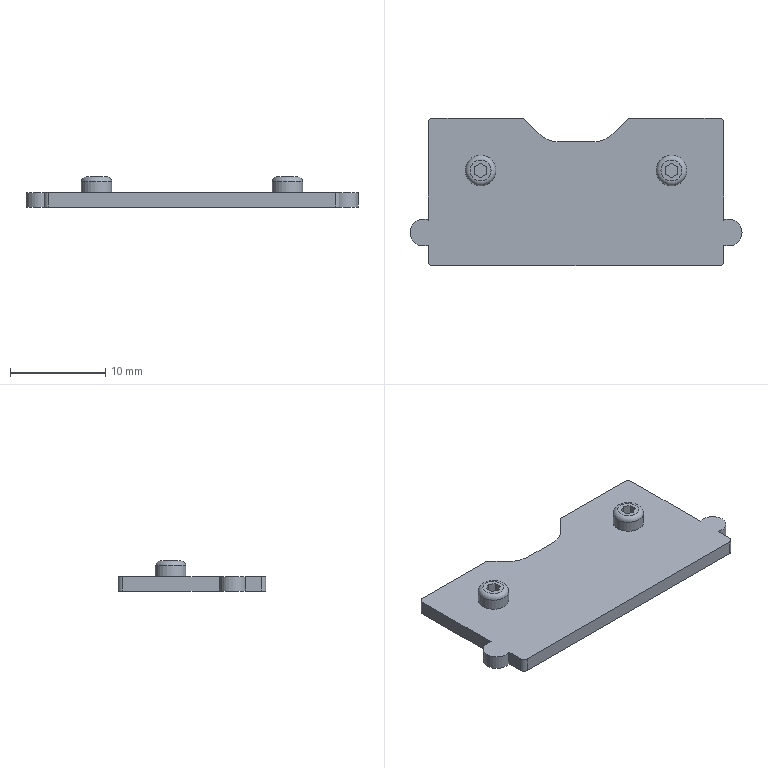Part | STEP file | BODY6_E-RAM6-S-640-ME30-C5 | 1 solid | 40 faces | box 34.8 x 15.5 x 3.15 mm | volume 724.972 mm3 | plane 28 | cylinder 10 | torus 2 | commonest cylinder face diameters 1 x4 2.8 x2 3.2 x2 6 x2
STEP:
#1=CARTESIAN_POINT('',(15.,5.5,1.5));
#2=VERTEX_POINT('',#1);
#3=CARTESIAN_POINT('',(5.5,5.5,1.5));
#4=VERTEX_POINT('',#3);
#5=CARTESIAN_POINT('',(-15.5,5.5,1.5));
#6=DIRECTION('',(-1.,0.,0.));
#7=VECTOR('',#6,1000.);
#8=LINE('',#5,#7);
#9=EDGE_CURVE('',#2,#4,#8,.T.);
#10=ORIENTED_EDGE('',*,*,#9,.F.);
#11=CARTESIAN_POINT('',(15.,5.5,0.));
#12=VERTEX_POINT('',#11);
#13=CARTESIAN_POINT('',(15.,5.5,1.5));
#14=DIRECTION('',(0.,0.,-1.));
#15=VECTOR('',#14,1000.);
#16=LINE('',#13,#15);
#17=EDGE_CURVE('',#2,#12,#16,.T.);
#18=ORIENTED_EDGE('',*,*,#17,.T.);
#19=CARTESIAN_POINT('',(5.5,5.5,0.));
#20=VERTEX_POINT('',#19);
#21=CARTESIAN_POINT('',(-15.5,5.5,0.));
#22=DIRECTION('',(-1.,0.,0.));
#23=VECTOR('',#22,1000.);
#24=LINE('',#21,#23);
#25=EDGE_CURVE('',#12,#20,#24,.T.);
#26=ORIENTED_EDGE('',*,*,#25,.T.);
#27=CARTESIAN_POINT('',(5.5,5.5,0.));
#28=DIRECTION('',(0.,0.,1.));
#29=VECTOR('',#28,1000.);
#30=LINE('',#27,#29);
#31=EDGE_CURVE('',#20,#4,#30,.T.);
#32=ORIENTED_EDGE('',*,*,#31,.T.);
#33=EDGE_LOOP('',(#10,#18,#26,#32));
#34=FACE_OUTER_BOUND('',#33,.T.);
#35=CARTESIAN_POINT('',(-15.5,5.5,1.5));
#36=DIRECTION('',(0.,-1.,0.));
#37=DIRECTION('',(0.,0.,-1.));
#38=AXIS2_PLACEMENT_3D('',#35,#36,#37);
#39=PLANE('',#38);
#40=ADVANCED_FACE('',(#34),#39,.F.);
#41=CARTESIAN_POINT('',(-15.5,-7.808,0.));
#42=VERTEX_POINT('',#41);
#43=CARTESIAN_POINT('',(-15.5,-9.5,0.));
#44=VERTEX_POINT('',#43);
#45=CARTESIAN_POINT('',(-15.5,-10.,0.));
#46=DIRECTION('',(0.,-1.,0.));
#47=VECTOR('',#46,1000.);
#48=LINE('',#45,#47);
#49=EDGE_CURVE('',#42,#44,#48,.T.);
#50=ORIENTED_EDGE('',*,*,#49,.T.);
#51=CARTESIAN_POINT('',(-15.5,-9.5,1.5));
#52=VERTEX_POINT('',#51);
#53=CARTESIAN_POINT('',(-15.5,-9.5,1.5));
#54=DIRECTION('',(0.,0.,1.));
#55=VECTOR('',#54,1000.);
#56=LINE('',#53,#55);
#57=EDGE_CURVE('',#44,#52,#56,.T.);
#58=ORIENTED_EDGE('',*,*,#57,.T.);
#59=CARTESIAN_POINT('',(-15.5,-7.808,1.5));
#60=VERTEX_POINT('',#59);
#61=CARTESIAN_POINT('',(-15.5,-10.,1.5));
#62=DIRECTION('',(0.,-1.,0.));
#63=VECTOR('',#62,1000.);
#64=LINE('',#61,#63);
#65=EDGE_CURVE('',#60,#52,#64,.T.);
#66=ORIENTED_EDGE('',*,*,#65,.F.);
#67=CARTESIAN_POINT('',(-15.5,-7.808,1.5));
#68=DIRECTION('',(0.,0.,-1.));
#69=VECTOR('',#68,1000.);
#70=LINE('',#67,#69);
#71=EDGE_CURVE('',#60,#42,#70,.T.);
#72=ORIENTED_EDGE('',*,*,#71,.T.);
#73=EDGE_LOOP('',(#50,#58,#66,#72));
#74=FACE_OUTER_BOUND('',#73,.T.);
#75=CARTESIAN_POINT('',(-15.5,-10.,1.5));
#76=DIRECTION('',(1.,0.,0.));
#77=DIRECTION('',(0.,0.,-1.));
#78=AXIS2_PLACEMENT_3D('',#75,#76,#77);
#79=PLANE('',#78);
#80=ADVANCED_FACE('',(#74),#79,.F.);
#81=CARTESIAN_POINT('',(-15.,-10.,0.));
#82=VERTEX_POINT('',#81);
#83=CARTESIAN_POINT('',(15.,-10.,0.));
#84=VERTEX_POINT('',#83);
#85=CARTESIAN_POINT('',(-15.5,-10.,0.));
#86=DIRECTION('',(1.,0.,0.));
#87=VECTOR('',#86,1000.);
#88=LINE('',#85,#87);
#89=EDGE_CURVE('',#82,#84,#88,.T.);
#90=ORIENTED_EDGE('',*,*,#89,.T.);
#91=CARTESIAN_POINT('',(15.,-10.,1.5));
#92=VERTEX_POINT('',#91);
#93=CARTESIAN_POINT('',(15.,-10.,1.5));
#94=DIRECTION('',(0.,0.,1.));
#95=VECTOR('',#94,1000.);
#96=LINE('',#93,#95);
#97=EDGE_CURVE('',#84,#92,#96,.T.);
#98=ORIENTED_EDGE('',*,*,#97,.T.);
#99=CARTESIAN_POINT('',(-15.,-10.,1.5));
#100=VERTEX_POINT('',#99);
#101=CARTESIAN_POINT('',(-15.5,-10.,1.5));
#102=DIRECTION('',(1.,0.,0.));
#103=VECTOR('',#102,1000.);
#104=LINE('',#101,#103);
#105=EDGE_CURVE('',#100,#92,#104,.T.);
#106=ORIENTED_EDGE('',*,*,#105,.F.);
#107=CARTESIAN_POINT('',(-15.,-10.,1.5));
#108=DIRECTION('',(0.,0.,-1.));
#109=VECTOR('',#108,1000.);
#110=LINE('',#107,#109);
#111=EDGE_CURVE('',#100,#82,#110,.T.);
#112=ORIENTED_EDGE('',*,*,#111,.T.);
#113=EDGE_LOOP('',(#90,#98,#106,#112));
#114=FACE_OUTER_BOUND('',#113,.T.);
#115=CARTESIAN_POINT('',(-15.5,-10.,1.5));
#116=DIRECTION('',(0.,1.,0.));
#117=DIRECTION('',(0.,0.,1.));
#118=AXIS2_PLACEMENT_3D('',#115,#116,#117);
#119=PLANE('',#118);
#120=ADVANCED_FACE('',(#114),#119,.F.);
#121=CARTESIAN_POINT('',(15.5,-9.5,1.5));
#122=VERTEX_POINT('',#121);
#123=CARTESIAN_POINT('',(15.5,-7.808,1.5));
#124=VERTEX_POINT('',#123);
#125=CARTESIAN_POINT('',(15.5,-10.,1.5));
#126=DIRECTION('',(0.,1.,0.));
#127=VECTOR('',#126,1000.);
#128=LINE('',#125,#127);
#129=EDGE_CURVE('',#122,#124,#128,.T.);
#130=ORIENTED_EDGE('',*,*,#129,.F.);
#131=CARTESIAN_POINT('',(15.5,-9.5,0.));
#132=VERTEX_POINT('',#131);
#133=CARTESIAN_POINT('',(15.5,-9.5,1.5));
#134=DIRECTION('',(0.,0.,-1.));
#135=VECTOR('',#134,1000.);
#136=LINE('',#133,#135);
#137=EDGE_CURVE('',#122,#132,#136,.T.);
#138=ORIENTED_EDGE('',*,*,#137,.T.);
#139=CARTESIAN_POINT('',(15.5,-7.808,0.));
#140=VERTEX_POINT('',#139);
#141=CARTESIAN_POINT('',(15.5,-10.,0.));
#142=DIRECTION('',(0.,1.,0.));
#143=VECTOR('',#142,1000.);
#144=LINE('',#141,#143);
#145=EDGE_CURVE('',#132,#140,#144,.T.);
#146=ORIENTED_EDGE('',*,*,#145,.T.);
#147=CARTESIAN_POINT('',(15.5,-7.808,1.5));
#148=DIRECTION('',(0.,0.,-1.));
#149=VECTOR('',#148,1000.);
#150=LINE('',#147,#149);
#151=EDGE_CURVE('',#124,#140,#150,.T.);
#152=ORIENTED_EDGE('',*,*,#151,.F.);
#153=EDGE_LOOP('',(#130,#138,#146,#152));
#154=FACE_OUTER_BOUND('',#153,.T.);
#155=CARTESIAN_POINT('',(15.5,-10.,1.5));
#156=DIRECTION('',(-1.,0.,0.));
#157=DIRECTION('',(0.,0.,1.));
#158=AXIS2_PLACEMENT_3D('',#155,#156,#157);
#159=PLANE('',#158);
#160=ADVANCED_FACE('',(#154),#159,.F.);
#161=CARTESIAN_POINT('',(15.5,-5.192,0.));
#162=VERTEX_POINT('',#161);
#163=CARTESIAN_POINT('',(16.,-6.5,0.));
#164=DIRECTION('',(0.,0.,1.));
#165=DIRECTION('',(1.,0.,0.));
#166=AXIS2_PLACEMENT_3D('',#163,#164,#165);
#167=CIRCLE('',#166,1.4);
#168=EDGE_CURVE('',#140,#162,#167,.T.);
#169=ORIENTED_EDGE('',*,*,#168,.T.);
#170=CARTESIAN_POINT('',(15.5,-5.192,1.5));
#171=VERTEX_POINT('',#170);
#172=CARTESIAN_POINT('',(15.5,-5.192,1.5));
#173=DIRECTION('',(0.,0.,-1.));
#174=VECTOR('',#173,1000.);
#175=LINE('',#172,#174);
#176=EDGE_CURVE('',#171,#162,#175,.T.);
#177=ORIENTED_EDGE('',*,*,#176,.F.);
#178=CARTESIAN_POINT('',(16.,-6.5,1.5));
#179=DIRECTION('',(0.,0.,1.));
#180=DIRECTION('',(1.,0.,0.));
#181=AXIS2_PLACEMENT_3D('',#178,#179,#180);
#182=CIRCLE('',#181,1.4);
#183=EDGE_CURVE('',#124,#171,#182,.T.);
#184=ORIENTED_EDGE('',*,*,#183,.F.);
#185=ORIENTED_EDGE('',*,*,#151,.T.);
#186=EDGE_LOOP('',(#169,#177,#184,#185));
#187=FACE_OUTER_BOUND('',#186,.T.);
#188=CARTESIAN_POINT('',(16.,-6.5,1.5));
#189=DIRECTION('',(0.,0.,-1.));
#190=DIRECTION('',(1.,0.,0.));
#191=AXIS2_PLACEMENT_3D('',#188,#189,#190);
#192=CYLINDRICAL_SURFACE('',#191,1.4);
#193=ADVANCED_FACE('',(#187),#192,.T.);
#194=CARTESIAN_POINT('',(15.5,5.,0.));
#195=VERTEX_POINT('',#194);
#196=CARTESIAN_POINT('',(15.5,-5.192,0.));
#197=DIRECTION('',(0.,1.,0.));
#198=VECTOR('',#197,1000.);
#199=LINE('',#196,#198);
#200=EDGE_CURVE('',#162,#195,#199,.T.);
#201=ORIENTED_EDGE('',*,*,#200,.T.);
#202=CARTESIAN_POINT('',(15.5,5.,1.5));
#203=VERTEX_POINT('',#202);
#204=CARTESIAN_POINT('',(15.5,5.,1.5));
#205=DIRECTION('',(0.,0.,1.));
#206=VECTOR('',#205,1000.);
#207=LINE('',#204,#206);
#208=EDGE_CURVE('',#195,#203,#207,.T.);
#209=ORIENTED_EDGE('',*,*,#208,.T.);
#210=CARTESIAN_POINT('',(15.5,-5.192,1.5));
#211=DIRECTION('',(0.,1.,0.));
#212=VECTOR('',#211,1000.);
#213=LINE('',#210,#212);
#214=EDGE_CURVE('',#171,#203,#213,.T.);
#215=ORIENTED_EDGE('',*,*,#214,.F.);
#216=ORIENTED_EDGE('',*,*,#176,.T.);
#217=EDGE_LOOP('',(#201,#209,#215,#216));
#218=FACE_OUTER_BOUND('',#217,.T.);
#219=CARTESIAN_POINT('',(15.5,-5.192,1.5));
#220=DIRECTION('',(-1.,0.,0.));
#221=DIRECTION('',(0.,0.,1.));
#222=AXIS2_PLACEMENT_3D('',#219,#220,#221);
#223=PLANE('',#222);
#224=ADVANCED_FACE('',(#218),#223,.F.);
#225=CARTESIAN_POINT('',(-5.5,5.5,0.));
#226=VERTEX_POINT('',#225);
#227=CARTESIAN_POINT('',(-15.,5.5,0.));
#228=VERTEX_POINT('',#227);
#229=CARTESIAN_POINT('',(-15.5,5.5,0.));
#230=DIRECTION('',(-1.,0.,0.));
#231=VECTOR('',#230,1000.);
#232=LINE('',#229,#231);
#233=EDGE_CURVE('',#226,#228,#232,.T.);
#234=ORIENTED_EDGE('',*,*,#233,.T.);
#235=CARTESIAN_POINT('',(-15.,5.5,1.5));
#236=VERTEX_POINT('',#235);
#237=CARTESIAN_POINT('',(-15.,5.5,1.5));
#238=DIRECTION('',(0.,0.,1.));
#239=VECTOR('',#238,1000.);
#240=LINE('',#237,#239);
#241=EDGE_CURVE('',#228,#236,#240,.T.);
#242=ORIENTED_EDGE('',*,*,#241,.T.);
#243=CARTESIAN_POINT('',(-5.5,5.5,1.5));
#244=VERTEX_POINT('',#243);
#245=CARTESIAN_POINT('',(-15.5,5.5,1.5));
#246=DIRECTION('',(-1.,0.,0.));
#247=VECTOR('',#246,1000.);
#248=LINE('',#245,#247);
#249=EDGE_CURVE('',#244,#236,#248,.T.);
#250=ORIENTED_EDGE('',*,*,#249,.F.);
#251=CARTESIAN_POINT('',(-5.5,5.5,0.));
#252=DIRECTION('',(0.,0.,1.));
#253=VECTOR('',#252,1000.);
#254=LINE('',#251,#253);
#255=EDGE_CURVE('',#226,#244,#254,.T.);
#256=ORIENTED_EDGE('',*,*,#255,.F.);
#257=EDGE_LOOP('',(#234,#242,#250,#256));
#258=FACE_OUTER_BOUND('',#257,.T.);
#259=CARTESIAN_POINT('',(-15.5,5.5,1.5));
#260=DIRECTION('',(0.,-1.,0.));
#261=DIRECTION('',(0.,0.,-1.));
#262=AXIS2_PLACEMENT_3D('',#259,#260,#261);
#263=PLANE('',#262);
#264=ADVANCED_FACE('',(#258),#263,.F.);
#265=CARTESIAN_POINT('',(-15.5,5.,1.5));
#266=VERTEX_POINT('',#265);
#267=CARTESIAN_POINT('',(-15.5,-5.192,1.5));
#268=VERTEX_POINT('',#267);
#269=CARTESIAN_POINT('',(-15.5,-5.192,1.5));
#270=DIRECTION('',(0.,-1.,0.));
#271=VECTOR('',#270,1000.);
#272=LINE('',#269,#271);
#273=EDGE_CURVE('',#266,#268,#272,.T.);
#274=ORIENTED_EDGE('',*,*,#273,.F.);
#275=CARTESIAN_POINT('',(-15.5,5.,0.));
#276=VERTEX_POINT('',#275);
#277=CARTESIAN_POINT('',(-15.5,5.,1.5));
#278=DIRECTION('',(0.,0.,-1.));
#279=VECTOR('',#278,1000.);
#280=LINE('',#277,#279);
#281=EDGE_CURVE('',#266,#276,#280,.T.);
#282=ORIENTED_EDGE('',*,*,#281,.T.);
#283=CARTESIAN_POINT('',(-15.5,-5.192,0.));
#284=VERTEX_POINT('',#283);
#285=CARTESIAN_POINT('',(-15.5,-5.192,0.));
#286=DIRECTION('',(0.,-1.,0.));
#287=VECTOR('',#286,1000.);
#288=LINE('',#285,#287);
#289=EDGE_CURVE('',#276,#284,#288,.T.);
#290=ORIENTED_EDGE('',*,*,#289,.T.);
#291=CARTESIAN_POINT('',(-15.5,-5.192,1.5));
#292=DIRECTION('',(0.,0.,-1.));
#293=VECTOR('',#292,1000.);
#294=LINE('',#291,#293);
#295=EDGE_CURVE('',#268,#284,#294,.T.);
#296=ORIENTED_EDGE('',*,*,#295,.F.);
#297=EDGE_LOOP('',(#274,#282,#290,#296));
#298=FACE_OUTER_BOUND('',#297,.T.);
#299=CARTESIAN_POINT('',(-15.5,-5.192,1.5));
#300=DIRECTION('',(1.,0.,0.));
#301=DIRECTION('',(0.,0.,-1.));
#302=AXIS2_PLACEMENT_3D('',#299,#300,#301);
#303=PLANE('',#302);
#304=ADVANCED_FACE('',(#298),#303,.F.);
#305=CARTESIAN_POINT('',(-16.,-6.5,0.));
#306=DIRECTION('',(0.,0.,1.));
#307=DIRECTION('',(1.,0.,0.));
#308=AXIS2_PLACEMENT_3D('',#305,#306,#307);
#309=CIRCLE('',#308,1.4);
#310=EDGE_CURVE('',#284,#42,#309,.T.);
#311=ORIENTED_EDGE('',*,*,#310,.T.);
#312=ORIENTED_EDGE('',*,*,#71,.F.);
#313=CARTESIAN_POINT('',(-16.,-6.5,1.5));
#314=DIRECTION('',(0.,0.,1.));
#315=DIRECTION('',(1.,0.,0.));
#316=AXIS2_PLACEMENT_3D('',#313,#314,#315);
#317=CIRCLE('',#316,1.4);
#318=EDGE_CURVE('',#268,#60,#317,.T.);
#319=ORIENTED_EDGE('',*,*,#318,.F.);
#320=ORIENTED_EDGE('',*,*,#295,.T.);
#321=EDGE_LOOP('',(#311,#312,#319,#320));
#322=FACE_OUTER_BOUND('',#321,.T.);
#323=CARTESIAN_POINT('',(-16.,-6.5,1.5));
#324=DIRECTION('',(0.,0.,-1.));
#325=DIRECTION('',(-1.,0.,0.));
#326=AXIS2_PLACEMENT_3D('',#323,#324,#325);
#327=CYLINDRICAL_SURFACE('',#326,1.4);
#328=ADVANCED_FACE('',(#322),#327,.T.);
#329=ORIENTED_EDGE('',*,*,#105,.T.);
#330=CARTESIAN_POINT('',(15.,-9.5,1.5));
#331=DIRECTION('',(0.,0.,1.));
#332=DIRECTION('',(1.,0.,0.));
#333=AXIS2_PLACEMENT_3D('',#330,#331,#332);
#334=CIRCLE('',#333,0.5);
#335=EDGE_CURVE('',#92,#122,#334,.T.);
#336=ORIENTED_EDGE('',*,*,#335,.T.);
#337=ORIENTED_EDGE('',*,*,#129,.T.);
#338=ORIENTED_EDGE('',*,*,#183,.T.);
#339=ORIENTED_EDGE('',*,*,#214,.T.);
#340=CARTESIAN_POINT('',(15.,5.,1.5));
#341=DIRECTION('',(0.,0.,1.));
#342=DIRECTION('',(1.,0.,0.));
#343=AXIS2_PLACEMENT_3D('',#340,#341,#342);
#344=CIRCLE('',#343,0.5);
#345=EDGE_CURVE('',#203,#2,#344,.T.);
#346=ORIENTED_EDGE('',*,*,#345,.T.);
#347=ORIENTED_EDGE('',*,*,#9,.T.);
#348=CARTESIAN_POINT('',(3.879,3.879,1.5));
#349=VERTEX_POINT('',#348);
#350=CARTESIAN_POINT('',(3.,3.,1.5));
#351=DIRECTION('',(0.7071,0.7071,0.));
#352=VECTOR('',#351,1000.);
#353=LINE('',#350,#352);
#354=EDGE_CURVE('',#349,#4,#353,.T.);
#355=ORIENTED_EDGE('',*,*,#354,.F.);
#356=CARTESIAN_POINT('',(1.757,3.,1.5));
#357=VERTEX_POINT('',#356);
#358=CARTESIAN_POINT('',(1.757,6.,1.5));
#359=DIRECTION('',(0.,0.,-1.));
#360=DIRECTION('',(1.,0.,0.));
#361=AXIS2_PLACEMENT_3D('',#358,#359,#360);
#362=CIRCLE('',#361,3.);
#363=EDGE_CURVE('',#349,#357,#362,.T.);
#364=ORIENTED_EDGE('',*,*,#363,.T.);
#365=CARTESIAN_POINT('',(-1.757,3.,1.5));
#366=VERTEX_POINT('',#365);
#367=CARTESIAN_POINT('',(-3.,3.,1.5));
#368=DIRECTION('',(1.,0.,0.));
#369=VECTOR('',#368,1000.);
#370=LINE('',#367,#369);
#371=EDGE_CURVE('',#366,#357,#370,.T.);
#372=ORIENTED_EDGE('',*,*,#371,.F.);
#373=CARTESIAN_POINT('',(-3.879,3.879,1.5));
#374=VERTEX_POINT('',#373);
#375=CARTESIAN_POINT('',(-1.757,6.,1.5));
#376=DIRECTION('',(0.,0.,-1.));
#377=DIRECTION('',(1.,0.,0.));
#378=AXIS2_PLACEMENT_3D('',#375,#376,#377);
#379=CIRCLE('',#378,3.);
#380=EDGE_CURVE('',#366,#374,#379,.T.);
#381=ORIENTED_EDGE('',*,*,#380,.T.);
#382=CARTESIAN_POINT('',(-5.5,5.5,1.5));
#383=DIRECTION('',(0.7071,-0.7071,0.));
#384=VECTOR('',#383,1000.);
#385=LINE('',#382,#384);
#386=EDGE_CURVE('',#244,#374,#385,.T.);
#387=ORIENTED_EDGE('',*,*,#386,.F.);
#388=ORIENTED_EDGE('',*,*,#249,.T.);
#389=CARTESIAN_POINT('',(-15.,5.,1.5));
#390=DIRECTION('',(0.,0.,1.));
#391=DIRECTION('',(1.,0.,0.));
#392=AXIS2_PLACEMENT_3D('',#389,#390,#391);
#393=CIRCLE('',#392,0.5);
#394=EDGE_CURVE('',#236,#266,#393,.T.);
#395=ORIENTED_EDGE('',*,*,#394,.T.);
#396=ORIENTED_EDGE('',*,*,#273,.T.);
#397=ORIENTED_EDGE('',*,*,#318,.T.);
#398=ORIENTED_EDGE('',*,*,#65,.T.);
#399=CARTESIAN_POINT('',(-15.,-9.5,1.5));
#400=DIRECTION('',(0.,0.,1.));
#401=DIRECTION('',(1.,0.,0.));
#402=AXIS2_PLACEMENT_3D('',#399,#400,#401);
#403=CIRCLE('',#402,0.5);
#404=EDGE_CURVE('',#52,#100,#403,.T.);
#405=ORIENTED_EDGE('',*,*,#404,.T.);
#406=EDGE_LOOP('',(#329,#336,#337,#338,#339,#346,#347,#355,#364,#372,#381,#387,#388,#395,#396,#397,#398,#405));
#407=FACE_OUTER_BOUND('',#406,.T.);
#408=CARTESIAN_POINT('',(11.6,0.,1.5));
#409=VERTEX_POINT('',#408);
#410=CARTESIAN_POINT('',(10.,0.,1.5));
#411=DIRECTION('',(0.,0.,1.));
#412=DIRECTION('',(1.,0.,0.));
#413=AXIS2_PLACEMENT_3D('',#410,#411,#412);
#414=CIRCLE('',#413,1.6);
#415=EDGE_CURVE('',#409,#409,#414,.T.);
#416=ORIENTED_EDGE('',*,*,#415,.F.);
#417=EDGE_LOOP('',(#416));
#418=FACE_BOUND('',#417,.T.);
#419=CARTESIAN_POINT('',(-8.4,0.,1.5));
#420=VERTEX_POINT('',#419);
#421=CARTESIAN_POINT('',(-10.,0.,1.5));
#422=DIRECTION('',(0.,0.,1.));
#423=DIRECTION('',(1.,0.,0.));
#424=AXIS2_PLACEMENT_3D('',#421,#422,#423);
#425=CIRCLE('',#424,1.6);
#426=EDGE_CURVE('',#420,#420,#425,.T.);
#427=ORIENTED_EDGE('',*,*,#426,.F.);
#428=EDGE_LOOP('',(#427));
#429=FACE_BOUND('',#428,.T.);
#430=CARTESIAN_POINT('',(-16.,-6.5,1.5));
#431=DIRECTION('',(0.,0.,1.));
#432=DIRECTION('',(1.,0.,0.));
#433=AXIS2_PLACEMENT_3D('',#430,#431,#432);
#434=PLANE('',#433);
#435=ADVANCED_FACE('',(#407,#418,#429),#434,.T.);
#436=ORIENTED_EDGE('',*,*,#145,.F.);
#437=CARTESIAN_POINT('',(15.,-9.5,0.));
#438=DIRECTION('',(0.,0.,-1.));
#439=DIRECTION('',(1.,0.,0.));
#440=AXIS2_PLACEMENT_3D('',#437,#438,#439);
#441=CIRCLE('',#440,0.5);
#442=EDGE_CURVE('',#132,#84,#441,.T.);
#443=ORIENTED_EDGE('',*,*,#442,.T.);
#444=ORIENTED_EDGE('',*,*,#89,.F.);
#445=CARTESIAN_POINT('',(-15.,-9.5,0.));
#446=DIRECTION('',(0.,0.,-1.));
#447=DIRECTION('',(1.,0.,0.));
#448=AXIS2_PLACEMENT_3D('',#445,#446,#447);
#449=CIRCLE('',#448,0.5);
#450=EDGE_CURVE('',#82,#44,#449,.T.);
#451=ORIENTED_EDGE('',*,*,#450,.T.);
#452=ORIENTED_EDGE('',*,*,#49,.F.);
#453=ORIENTED_EDGE('',*,*,#310,.F.);
#454=ORIENTED_EDGE('',*,*,#289,.F.);
#455=CARTESIAN_POINT('',(-15.,5.,0.));
#456=DIRECTION('',(0.,0.,-1.));
#457=DIRECTION('',(1.,0.,0.));
#458=AXIS2_PLACEMENT_3D('',#455,#456,#457);
#459=CIRCLE('',#458,0.5);
#460=EDGE_CURVE('',#276,#228,#459,.T.);
#461=ORIENTED_EDGE('',*,*,#460,.T.);
#462=ORIENTED_EDGE('',*,*,#233,.F.);
#463=CARTESIAN_POINT('',(-3.879,3.879,0.));
#464=VERTEX_POINT('',#463);
#465=CARTESIAN_POINT('',(-5.5,5.5,0.));
#466=DIRECTION('',(0.7071,-0.7071,0.));
#467=VECTOR('',#466,1000.);
#468=LINE('',#465,#467);
#469=EDGE_CURVE('',#226,#464,#468,.T.);
#470=ORIENTED_EDGE('',*,*,#469,.T.);
#471=CARTESIAN_POINT('',(-1.757,3.,0.));
#472=VERTEX_POINT('',#471);
#473=CARTESIAN_POINT('',(-1.757,6.,0.));
#474=DIRECTION('',(0.,0.,1.));
#475=DIRECTION('',(1.,0.,0.));
#476=AXIS2_PLACEMENT_3D('',#473,#474,#475);
#477=CIRCLE('',#476,3.);
#478=EDGE_CURVE('',#464,#472,#477,.T.);
#479=ORIENTED_EDGE('',*,*,#478,.T.);
#480=CARTESIAN_POINT('',(1.757,3.,0.));
#481=VERTEX_POINT('',#480);
#482=CARTESIAN_POINT('',(-3.,3.,0.));
#483=DIRECTION('',(1.,0.,0.));
#484=VECTOR('',#483,1000.);
#485=LINE('',#482,#484);
#486=EDGE_CURVE('',#472,#481,#485,.T.);
#487=ORIENTED_EDGE('',*,*,#486,.T.);
#488=CARTESIAN_POINT('',(3.879,3.879,0.));
#489=VERTEX_POINT('',#488);
#490=CARTESIAN_POINT('',(1.757,6.,0.));
#491=DIRECTION('',(0.,0.,1.));
#492=DIRECTION('',(1.,0.,0.));
#493=AXIS2_PLACEMENT_3D('',#490,#491,#492);
#494=CIRCLE('',#493,3.);
#495=EDGE_CURVE('',#481,#489,#494,.T.);
#496=ORIENTED_EDGE('',*,*,#495,.T.);
#497=CARTESIAN_POINT('',(3.,3.,0.));
#498=DIRECTION('',(0.7071,0.7071,0.));
#499=VECTOR('',#498,1000.);
#500=LINE('',#497,#499);
#501=EDGE_CURVE('',#489,#20,#500,.T.);
#502=ORIENTED_EDGE('',*,*,#501,.T.);
#503=ORIENTED_EDGE('',*,*,#25,.F.);
#504=CARTESIAN_POINT('',(15.,5.,0.));
#505=DIRECTION('',(0.,0.,-1.));
#506=DIRECTION('',(1.,0.,0.));
#507=AXIS2_PLACEMENT_3D('',#504,#505,#506);
#508=CIRCLE('',#507,0.5);
#509=EDGE_CURVE('',#12,#195,#508,.T.);
#510=ORIENTED_EDGE('',*,*,#509,.T.);
#511=ORIENTED_EDGE('',*,*,#200,.F.);
#512=ORIENTED_EDGE('',*,*,#168,.F.);
#513=EDGE_LOOP('',(#436,#443,#444,#451,#452,#453,#454,#461,#462,#470,#479,#487,#496,#502,#503,#510,#511,#512));
#514=FACE_OUTER_BOUND('',#513,.T.);
#515=CARTESIAN_POINT('',(-16.,-6.5,0.));
#516=DIRECTION('',(0.,0.,1.));
#517=DIRECTION('',(1.,0.,0.));
#518=AXIS2_PLACEMENT_3D('',#515,#516,#517);
#519=PLANE('',#518);
#520=ADVANCED_FACE('',(#514),#519,.F.);
#521=ORIENTED_EDGE('',*,*,#426,.T.);
#522=CARTESIAN_POINT('',(-8.4,0.,2.65));
#523=VERTEX_POINT('',#522);
#524=CARTESIAN_POINT('',(-8.4,0.,3.15));
#525=DIRECTION('',(0.,0.,1.));
#526=VECTOR('',#525,1.6);
#527=LINE('',#524,#526);
#528=EDGE_CURVE('',#420,#523,#527,.T.);
#529=ORIENTED_EDGE('',*,*,#528,.T.);
#530=CARTESIAN_POINT('',(-11.6,0.,2.65));
#531=VERTEX_POINT('',#530);
#532=CARTESIAN_POINT('',(-10.,0.,2.65));
#533=DIRECTION('',(0.,0.,-1.));
#534=DIRECTION('',(1.,0.,0.));
#535=AXIS2_PLACEMENT_3D('',#532,#533,#534);
#536=CIRCLE('',#535,1.6);
#537=EDGE_CURVE('',#523,#531,#536,.T.);
#538=ORIENTED_EDGE('',*,*,#537,.T.);
#539=CARTESIAN_POINT('',(-10.,0.,2.65));
#540=DIRECTION('',(0.,0.,-1.));
#541=DIRECTION('',(1.,0.,0.));
#542=AXIS2_PLACEMENT_3D('',#539,#540,#541);
#543=CIRCLE('',#542,1.6);
#544=EDGE_CURVE('',#531,#523,#543,.T.);
#545=ORIENTED_EDGE('',*,*,#544,.T.);
#546=ORIENTED_EDGE('',*,*,#528,.F.);
#547=EDGE_LOOP('',(#521,#529,#538,#545,#546));
#548=FACE_OUTER_BOUND('',#547,.T.);
#549=CARTESIAN_POINT('',(-10.,0.,3.15));
#550=DIRECTION('',(0.,0.,-1.));
#551=DIRECTION('',(-1.,0.,0.));
#552=AXIS2_PLACEMENT_3D('',#549,#550,#551);
#553=CYLINDRICAL_SURFACE('',#552,1.6);
#554=ADVANCED_FACE('',(#548),#553,.T.);
#555=CARTESIAN_POINT('',(-8.9,0.,3.15));
#556=VERTEX_POINT('',#555);
#557=CARTESIAN_POINT('',(-11.1,0.,3.15));
#558=VERTEX_POINT('',#557);
#559=CARTESIAN_POINT('',(-10.,0.,3.15));
#560=DIRECTION('',(0.,0.,1.));
#561=DIRECTION('',(1.,0.,0.));
#562=AXIS2_PLACEMENT_3D('',#559,#560,#561);
#563=CIRCLE('',#562,1.1);
#564=EDGE_CURVE('',#556,#558,#563,.T.);
#565=ORIENTED_EDGE('',*,*,#564,.T.);
#566=CARTESIAN_POINT('',(-10.,0.,3.15));
#567=DIRECTION('',(0.,0.,1.));
#568=DIRECTION('',(1.,0.,0.));
#569=AXIS2_PLACEMENT_3D('',#566,#567,#568);
#570=CIRCLE('',#569,1.1);
#571=EDGE_CURVE('',#558,#556,#570,.T.);
#572=ORIENTED_EDGE('',*,*,#571,.T.);
#573=EDGE_LOOP('',(#565,#572));
#574=FACE_OUTER_BOUND('',#573,.T.);
#575=CARTESIAN_POINT('',(-9.35,0.3753,3.15));
#576=VERTEX_POINT('',#575);
#577=CARTESIAN_POINT('',(-10.,0.7506,3.15));
#578=VERTEX_POINT('',#577);
#579=CARTESIAN_POINT('',(-9.35,0.3753,3.15));
#580=DIRECTION('',(-0.866,0.5,0.));
#581=VECTOR('',#580,1000.);
#582=LINE('',#579,#581);
#583=EDGE_CURVE('',#576,#578,#582,.T.);
#584=ORIENTED_EDGE('',*,*,#583,.F.);
#585=CARTESIAN_POINT('',(-9.35,-0.3753,3.15));
#586=VERTEX_POINT('',#585);
#587=CARTESIAN_POINT('',(-9.35,-0.3753,3.15));
#588=DIRECTION('',(0.,1.,0.));
#589=VECTOR('',#588,1000.);
#590=LINE('',#587,#589);
#591=EDGE_CURVE('',#586,#576,#590,.T.);
#592=ORIENTED_EDGE('',*,*,#591,.F.);
#593=CARTESIAN_POINT('',(-10.,-0.7506,3.15));
#594=VERTEX_POINT('',#593);
#595=CARTESIAN_POINT('',(-10.,-0.7506,3.15));
#596=DIRECTION('',(0.866,0.5,0.));
#597=VECTOR('',#596,1000.);
#598=LINE('',#595,#597);
#599=EDGE_CURVE('',#594,#586,#598,.T.);
#600=ORIENTED_EDGE('',*,*,#599,.F.);
#601=CARTESIAN_POINT('',(-10.65,-0.3753,3.15));
#602=VERTEX_POINT('',#601);
#603=CARTESIAN_POINT('',(-10.65,-0.3753,3.15));
#604=DIRECTION('',(0.866,-0.5,0.));
#605=VECTOR('',#604,1000.);
#606=LINE('',#603,#605);
#607=EDGE_CURVE('',#602,#594,#606,.T.);
#608=ORIENTED_EDGE('',*,*,#607,.F.);
#609=CARTESIAN_POINT('',(-10.65,0.3753,3.15));
#610=VERTEX_POINT('',#609);
#611=CARTESIAN_POINT('',(-10.65,0.3753,3.15));
#612=DIRECTION('',(0.,-1.,0.));
#613=VECTOR('',#612,1000.);
#614=LINE('',#611,#613);
#615=EDGE_CURVE('',#610,#602,#614,.T.);
#616=ORIENTED_EDGE('',*,*,#615,.F.);
#617=CARTESIAN_POINT('',(-10.,0.7506,3.15));
#618=DIRECTION('',(-0.866,-0.5,0.));
#619=VECTOR('',#618,1000.);
#620=LINE('',#617,#619);
#621=EDGE_CURVE('',#578,#610,#620,.T.);
#622=ORIENTED_EDGE('',*,*,#621,.F.);
#623=EDGE_LOOP('',(#584,#592,#600,#608,#616,#622));
#624=FACE_BOUND('',#623,.T.);
#625=CARTESIAN_POINT('',(-10.,0.,3.15));
#626=DIRECTION('',(0.,0.,1.));
#627=DIRECTION('',(1.,0.,0.));
#628=AXIS2_PLACEMENT_3D('',#625,#626,#627);
#629=PLANE('',#628);
#630=ADVANCED_FACE('',(#574,#624),#629,.T.);
#631=ORIENTED_EDGE('',*,*,#415,.T.);
#632=CARTESIAN_POINT('',(11.6,0.,2.65));
#633=VERTEX_POINT('',#632);
#634=CARTESIAN_POINT('',(11.6,0.,3.15));
#635=DIRECTION('',(0.,0.,1.));
#636=VECTOR('',#635,1.6);
#637=LINE('',#634,#636);
#638=EDGE_CURVE('',#409,#633,#637,.T.);
#639=ORIENTED_EDGE('',*,*,#638,.T.);
#640=CARTESIAN_POINT('',(8.4,0.,2.65));
#641=VERTEX_POINT('',#640);
#642=CARTESIAN_POINT('',(10.,0.,2.65));
#643=DIRECTION('',(0.,0.,-1.));
#644=DIRECTION('',(1.,0.,0.));
#645=AXIS2_PLACEMENT_3D('',#642,#643,#644);
#646=CIRCLE('',#645,1.6);
#647=EDGE_CURVE('',#633,#641,#646,.T.);
#648=ORIENTED_EDGE('',*,*,#647,.T.);
#649=CARTESIAN_POINT('',(10.,0.,2.65));
#650=DIRECTION('',(0.,0.,-1.));
#651=DIRECTION('',(1.,0.,0.));
#652=AXIS2_PLACEMENT_3D('',#649,#650,#651);
#653=CIRCLE('',#652,1.6);
#654=EDGE_CURVE('',#641,#633,#653,.T.);
#655=ORIENTED_EDGE('',*,*,#654,.T.);
#656=ORIENTED_EDGE('',*,*,#638,.F.);
#657=EDGE_LOOP('',(#631,#639,#648,#655,#656));
#658=FACE_OUTER_BOUND('',#657,.T.);
#659=CARTESIAN_POINT('',(10.,0.,3.15));
#660=DIRECTION('',(0.,0.,-1.));
#661=DIRECTION('',(-1.,0.,0.));
#662=AXIS2_PLACEMENT_3D('',#659,#660,#661);
#663=CYLINDRICAL_SURFACE('',#662,1.6);
#664=ADVANCED_FACE('',(#658),#663,.T.);
#665=CARTESIAN_POINT('',(11.1,0.,3.15));
#666=VERTEX_POINT('',#665);
#667=CARTESIAN_POINT('',(8.9,0.,3.15));
#668=VERTEX_POINT('',#667);
#669=CARTESIAN_POINT('',(10.,0.,3.15));
#670=DIRECTION('',(0.,0.,1.));
#671=DIRECTION('',(1.,0.,0.));
#672=AXIS2_PLACEMENT_3D('',#669,#670,#671);
#673=CIRCLE('',#672,1.1);
#674=EDGE_CURVE('',#666,#668,#673,.T.);
#675=ORIENTED_EDGE('',*,*,#674,.T.);
#676=CARTESIAN_POINT('',(10.,0.,3.15));
#677=DIRECTION('',(0.,0.,1.));
#678=DIRECTION('',(1.,0.,0.));
#679=AXIS2_PLACEMENT_3D('',#676,#677,#678);
#680=CIRCLE('',#679,1.1);
#681=EDGE_CURVE('',#668,#666,#680,.T.);
#682=ORIENTED_EDGE('',*,*,#681,.T.);
#683=EDGE_LOOP('',(#675,#682));
#684=FACE_OUTER_BOUND('',#683,.T.);
#685=CARTESIAN_POINT('',(10.65,0.3753,3.15));
#686=VERTEX_POINT('',#685);
#687=CARTESIAN_POINT('',(10.,0.7506,3.15));
#688=VERTEX_POINT('',#687);
#689=CARTESIAN_POINT('',(10.65,0.3753,3.15));
#690=DIRECTION('',(-0.866,0.5,0.));
#691=VECTOR('',#690,1000.);
#692=LINE('',#689,#691);
#693=EDGE_CURVE('',#686,#688,#692,.T.);
#694=ORIENTED_EDGE('',*,*,#693,.F.);
#695=CARTESIAN_POINT('',(10.65,-0.3753,3.15));
#696=VERTEX_POINT('',#695);
#697=CARTESIAN_POINT('',(10.65,-0.3753,3.15));
#698=DIRECTION('',(0.,1.,0.));
#699=VECTOR('',#698,1000.);
#700=LINE('',#697,#699);
#701=EDGE_CURVE('',#696,#686,#700,.T.);
#702=ORIENTED_EDGE('',*,*,#701,.F.);
#703=CARTESIAN_POINT('',(10.,-0.7506,3.15));
#704=VERTEX_POINT('',#703);
#705=CARTESIAN_POINT('',(10.,-0.7506,3.15));
#706=DIRECTION('',(0.866,0.5,0.));
#707=VECTOR('',#706,1000.);
#708=LINE('',#705,#707);
#709=EDGE_CURVE('',#704,#696,#708,.T.);
#710=ORIENTED_EDGE('',*,*,#709,.F.);
#711=CARTESIAN_POINT('',(9.35,-0.3753,3.15));
#712=VERTEX_POINT('',#711);
#713=CARTESIAN_POINT('',(9.35,-0.3753,3.15));
#714=DIRECTION('',(0.866,-0.5,0.));
#715=VECTOR('',#714,1000.);
#716=LINE('',#713,#715);
#717=EDGE_CURVE('',#712,#704,#716,.T.);
#718=ORIENTED_EDGE('',*,*,#717,.F.);
#719=CARTESIAN_POINT('',(9.35,0.3753,3.15));
#720=VERTEX_POINT('',#719);
#721=CARTESIAN_POINT('',(9.35,0.3753,3.15));
#722=DIRECTION('',(0.,-1.,0.));
#723=VECTOR('',#722,1000.);
#724=LINE('',#721,#723);
#725=EDGE_CURVE('',#720,#712,#724,.T.);
#726=ORIENTED_EDGE('',*,*,#725,.F.);
#727=CARTESIAN_POINT('',(10.,0.7506,3.15));
#728=DIRECTION('',(-0.866,-0.5,0.));
#729=VECTOR('',#728,1000.);
#730=LINE('',#727,#729);
#731=EDGE_CURVE('',#688,#720,#730,.T.);
#732=ORIENTED_EDGE('',*,*,#731,.F.);
#733=EDGE_LOOP('',(#694,#702,#710,#718,#726,#732));
#734=FACE_BOUND('',#733,.T.);
#735=CARTESIAN_POINT('',(10.,0.,3.15));
#736=DIRECTION('',(0.,0.,1.));
#737=DIRECTION('',(1.,0.,0.));
#738=AXIS2_PLACEMENT_3D('',#735,#736,#737);
#739=PLANE('',#738);
#740=ADVANCED_FACE('',(#684,#734),#739,.T.);
#741=ORIENTED_EDGE('',*,*,#583,.T.);
#742=CARTESIAN_POINT('',(-10.,0.7506,2.11));
#743=VERTEX_POINT('',#742);
#744=CARTESIAN_POINT('',(-10.,0.7506,2.11));
#745=DIRECTION('',(0.,0.,1.));
#746=VECTOR('',#745,1000.);
#747=LINE('',#744,#746);
#748=EDGE_CURVE('',#743,#578,#747,.T.);
#749=ORIENTED_EDGE('',*,*,#748,.F.);
#750=CARTESIAN_POINT('',(-9.35,0.3753,2.11));
#751=VERTEX_POINT('',#750);
#752=CARTESIAN_POINT('',(-9.35,0.3753,2.11));
#753=DIRECTION('',(-0.866,0.5,0.));
#754=VECTOR('',#753,1000.);
#755=LINE('',#752,#754);
#756=EDGE_CURVE('',#751,#743,#755,.T.);
#757=ORIENTED_EDGE('',*,*,#756,.F.);
#758=CARTESIAN_POINT('',(-9.35,0.3753,2.11));
#759=DIRECTION('',(0.,0.,1.));
#760=VECTOR('',#759,1000.);
#761=LINE('',#758,#760);
#762=EDGE_CURVE('',#751,#576,#761,.T.);
#763=ORIENTED_EDGE('',*,*,#762,.T.);
#764=EDGE_LOOP('',(#741,#749,#757,#763));
#765=FACE_OUTER_BOUND('',#764,.T.);
#766=CARTESIAN_POINT('',(-9.35,0.3753,2.11));
#767=DIRECTION('',(0.5,0.866,0.));
#768=DIRECTION('',(-0.866,0.5,0.));
#769=AXIS2_PLACEMENT_3D('',#766,#767,#768);
#770=PLANE('',#769);
#771=ADVANCED_FACE('',(#765),#770,.F.);
#772=ORIENTED_EDGE('',*,*,#591,.T.);
#773=ORIENTED_EDGE('',*,*,#762,.F.);
#774=CARTESIAN_POINT('',(-9.35,-0.3753,2.11));
#775=VERTEX_POINT('',#774);
#776=CARTESIAN_POINT('',(-9.35,-0.3753,2.11));
#777=DIRECTION('',(0.,1.,0.));
#778=VECTOR('',#777,1000.);
#779=LINE('',#776,#778);
#780=EDGE_CURVE('',#775,#751,#779,.T.);
#781=ORIENTED_EDGE('',*,*,#780,.F.);
#782=CARTESIAN_POINT('',(-9.35,-0.3753,2.11));
#783=DIRECTION('',(0.,0.,1.));
#784=VECTOR('',#783,1000.);
#785=LINE('',#782,#784);
#786=EDGE_CURVE('',#775,#586,#785,.T.);
#787=ORIENTED_EDGE('',*,*,#786,.T.);
#788=EDGE_LOOP('',(#772,#773,#781,#787));
#789=FACE_OUTER_BOUND('',#788,.T.);
#790=CARTESIAN_POINT('',(-9.35,-0.3753,2.11));
#791=DIRECTION('',(1.,0.,0.));
#792=DIRECTION('',(0.,0.,-1.));
#793=AXIS2_PLACEMENT_3D('',#790,#791,#792);
#794=PLANE('',#793);
#795=ADVANCED_FACE('',(#789),#794,.F.);
#796=ORIENTED_EDGE('',*,*,#599,.T.);
#797=ORIENTED_EDGE('',*,*,#786,.F.);
#798=CARTESIAN_POINT('',(-10.,-0.7506,2.11));
#799=VERTEX_POINT('',#798);
#800=CARTESIAN_POINT('',(-10.,-0.7506,2.11));
#801=DIRECTION('',(0.866,0.5,0.));
#802=VECTOR('',#801,1000.);
#803=LINE('',#800,#802);
#804=EDGE_CURVE('',#799,#775,#803,.T.);
#805=ORIENTED_EDGE('',*,*,#804,.F.);
#806=CARTESIAN_POINT('',(-10.,-0.7506,2.11));
#807=DIRECTION('',(0.,0.,1.));
#808=VECTOR('',#807,1000.);
#809=LINE('',#806,#808);
#810=EDGE_CURVE('',#799,#594,#809,.T.);
#811=ORIENTED_EDGE('',*,*,#810,.T.);
#812=EDGE_LOOP('',(#796,#797,#805,#811));
#813=FACE_OUTER_BOUND('',#812,.T.);
#814=CARTESIAN_POINT('',(-10.,-0.7506,2.11));
#815=DIRECTION('',(0.5,-0.866,0.));
#816=DIRECTION('',(0.866,0.5,0.));
#817=AXIS2_PLACEMENT_3D('',#814,#815,#816);
#818=PLANE('',#817);
#819=ADVANCED_FACE('',(#813),#818,.F.);
#820=ORIENTED_EDGE('',*,*,#607,.T.);
#821=ORIENTED_EDGE('',*,*,#810,.F.);
#822=CARTESIAN_POINT('',(-10.65,-0.3753,2.11));
#823=VERTEX_POINT('',#822);
#824=CARTESIAN_POINT('',(-10.65,-0.3753,2.11));
#825=DIRECTION('',(0.866,-0.5,0.));
#826=VECTOR('',#825,1000.);
#827=LINE('',#824,#826);
#828=EDGE_CURVE('',#823,#799,#827,.T.);
#829=ORIENTED_EDGE('',*,*,#828,.F.);
#830=CARTESIAN_POINT('',(-10.65,-0.3753,2.11));
#831=DIRECTION('',(0.,0.,1.));
#832=VECTOR('',#831,1000.);
#833=LINE('',#830,#832);
#834=EDGE_CURVE('',#823,#602,#833,.T.);
#835=ORIENTED_EDGE('',*,*,#834,.T.);
#836=EDGE_LOOP('',(#820,#821,#829,#835));
#837=FACE_OUTER_BOUND('',#836,.T.);
#838=CARTESIAN_POINT('',(-10.65,-0.3753,2.11));
#839=DIRECTION('',(-0.5,-0.866,0.));
#840=DIRECTION('',(0.866,-0.5,0.));
#841=AXIS2_PLACEMENT_3D('',#838,#839,#840);
#842=PLANE('',#841);
#843=ADVANCED_FACE('',(#837),#842,.F.);
#844=ORIENTED_EDGE('',*,*,#615,.T.);
#845=ORIENTED_EDGE('',*,*,#834,.F.);
#846=CARTESIAN_POINT('',(-10.65,0.3753,2.11));
#847=VERTEX_POINT('',#846);
#848=CARTESIAN_POINT('',(-10.65,0.3753,2.11));
#849=DIRECTION('',(0.,-1.,0.));
#850=VECTOR('',#849,1000.);
#851=LINE('',#848,#850);
#852=EDGE_CURVE('',#847,#823,#851,.T.);
#853=ORIENTED_EDGE('',*,*,#852,.F.);
#854=CARTESIAN_POINT('',(-10.65,0.3753,2.11));
#855=DIRECTION('',(0.,0.,1.));
#856=VECTOR('',#855,1000.);
#857=LINE('',#854,#856);
#858=EDGE_CURVE('',#847,#610,#857,.T.);
#859=ORIENTED_EDGE('',*,*,#858,.T.);
#860=EDGE_LOOP('',(#844,#845,#853,#859));
#861=FACE_OUTER_BOUND('',#860,.T.);
#862=CARTESIAN_POINT('',(-10.65,0.3753,2.11));
#863=DIRECTION('',(-1.,0.,0.));
#864=DIRECTION('',(0.,0.,1.));
#865=AXIS2_PLACEMENT_3D('',#862,#863,#864);
#866=PLANE('',#865);
#867=ADVANCED_FACE('',(#861),#866,.F.);
#868=ORIENTED_EDGE('',*,*,#621,.T.);
#869=ORIENTED_EDGE('',*,*,#858,.F.);
#870=CARTESIAN_POINT('',(-10.,0.7506,2.11));
#871=DIRECTION('',(-0.866,-0.5,0.));
#872=VECTOR('',#871,1000.);
#873=LINE('',#870,#872);
#874=EDGE_CURVE('',#743,#847,#873,.T.);
#875=ORIENTED_EDGE('',*,*,#874,.F.);
#876=ORIENTED_EDGE('',*,*,#748,.T.);
#877=EDGE_LOOP('',(#868,#869,#875,#876));
#878=FACE_OUTER_BOUND('',#877,.T.);
#879=CARTESIAN_POINT('',(-10.,0.7506,2.11));
#880=DIRECTION('',(-0.5,0.866,0.));
#881=DIRECTION('',(-0.866,-0.5,0.));
#882=AXIS2_PLACEMENT_3D('',#879,#880,#881);
#883=PLANE('',#882);
#884=ADVANCED_FACE('',(#878),#883,.F.);
#885=ORIENTED_EDGE('',*,*,#756,.T.);
#886=ORIENTED_EDGE('',*,*,#874,.T.);
#887=ORIENTED_EDGE('',*,*,#852,.T.);
#888=ORIENTED_EDGE('',*,*,#828,.T.);
#889=ORIENTED_EDGE('',*,*,#804,.T.);
#890=ORIENTED_EDGE('',*,*,#780,.T.);
#891=EDGE_LOOP('',(#885,#886,#887,#888,#889,#890));
#892=FACE_OUTER_BOUND('',#891,.T.);
#893=CARTESIAN_POINT('',(0.,0.,2.11));
#894=DIRECTION('',(0.,0.,1.));
#895=DIRECTION('',(1.,0.,0.));
#896=AXIS2_PLACEMENT_3D('',#893,#894,#895);
#897=PLANE('',#896);
#898=ADVANCED_FACE('',(#892),#897,.T.);
#899=ORIENTED_EDGE('',*,*,#693,.T.);
#900=CARTESIAN_POINT('',(10.,0.7506,2.11));
#901=VERTEX_POINT('',#900);
#902=CARTESIAN_POINT('',(10.,0.7506,2.11));
#903=DIRECTION('',(0.,0.,1.));
#904=VECTOR('',#903,1000.);
#905=LINE('',#902,#904);
#906=EDGE_CURVE('',#901,#688,#905,.T.);
#907=ORIENTED_EDGE('',*,*,#906,.F.);
#908=CARTESIAN_POINT('',(10.65,0.3753,2.11));
#909=VERTEX_POINT('',#908);
#910=CARTESIAN_POINT('',(10.65,0.3753,2.11));
#911=DIRECTION('',(-0.866,0.5,0.));
#912=VECTOR('',#911,1000.);
#913=LINE('',#910,#912);
#914=EDGE_CURVE('',#909,#901,#913,.T.);
#915=ORIENTED_EDGE('',*,*,#914,.F.);
#916=CARTESIAN_POINT('',(10.65,0.3753,2.11));
#917=DIRECTION('',(0.,0.,1.));
#918=VECTOR('',#917,1000.);
#919=LINE('',#916,#918);
#920=EDGE_CURVE('',#909,#686,#919,.T.);
#921=ORIENTED_EDGE('',*,*,#920,.T.);
#922=EDGE_LOOP('',(#899,#907,#915,#921));
#923=FACE_OUTER_BOUND('',#922,.T.);
#924=CARTESIAN_POINT('',(10.65,0.3753,2.11));
#925=DIRECTION('',(0.5,0.866,0.));
#926=DIRECTION('',(-0.866,0.5,0.));
#927=AXIS2_PLACEMENT_3D('',#924,#925,#926);
#928=PLANE('',#927);
#929=ADVANCED_FACE('',(#923),#928,.F.);
#930=ORIENTED_EDGE('',*,*,#701,.T.);
#931=ORIENTED_EDGE('',*,*,#920,.F.);
#932=CARTESIAN_POINT('',(10.65,-0.3753,2.11));
#933=VERTEX_POINT('',#932);
#934=CARTESIAN_POINT('',(10.65,-0.3753,2.11));
#935=DIRECTION('',(0.,1.,0.));
#936=VECTOR('',#935,1000.);
#937=LINE('',#934,#936);
#938=EDGE_CURVE('',#933,#909,#937,.T.);
#939=ORIENTED_EDGE('',*,*,#938,.F.);
#940=CARTESIAN_POINT('',(10.65,-0.3753,2.11));
#941=DIRECTION('',(0.,0.,1.));
#942=VECTOR('',#941,1000.);
#943=LINE('',#940,#942);
#944=EDGE_CURVE('',#933,#696,#943,.T.);
#945=ORIENTED_EDGE('',*,*,#944,.T.);
#946=EDGE_LOOP('',(#930,#931,#939,#945));
#947=FACE_OUTER_BOUND('',#946,.T.);
#948=CARTESIAN_POINT('',(10.65,-0.3753,2.11));
#949=DIRECTION('',(1.,0.,0.));
#950=DIRECTION('',(0.,0.,-1.));
#951=AXIS2_PLACEMENT_3D('',#948,#949,#950);
#952=PLANE('',#951);
#953=ADVANCED_FACE('',(#947),#952,.F.);
#954=ORIENTED_EDGE('',*,*,#709,.T.);
#955=ORIENTED_EDGE('',*,*,#944,.F.);
#956=CARTESIAN_POINT('',(10.,-0.7506,2.11));
#957=VERTEX_POINT('',#956);
#958=CARTESIAN_POINT('',(10.,-0.7506,2.11));
#959=DIRECTION('',(0.866,0.5,0.));
#960=VECTOR('',#959,1000.);
#961=LINE('',#958,#960);
#962=EDGE_CURVE('',#957,#933,#961,.T.);
#963=ORIENTED_EDGE('',*,*,#962,.F.);
#964=CARTESIAN_POINT('',(10.,-0.7506,2.11));
#965=DIRECTION('',(0.,0.,1.));
#966=VECTOR('',#965,1000.);
#967=LINE('',#964,#966);
#968=EDGE_CURVE('',#957,#704,#967,.T.);
#969=ORIENTED_EDGE('',*,*,#968,.T.);
#970=EDGE_LOOP('',(#954,#955,#963,#969));
#971=FACE_OUTER_BOUND('',#970,.T.);
#972=CARTESIAN_POINT('',(10.,-0.7506,2.11));
#973=DIRECTION('',(0.5,-0.866,0.));
#974=DIRECTION('',(0.866,0.5,0.));
#975=AXIS2_PLACEMENT_3D('',#972,#973,#974);
#976=PLANE('',#975);
#977=ADVANCED_FACE('',(#971),#976,.F.);
#978=ORIENTED_EDGE('',*,*,#717,.T.);
#979=ORIENTED_EDGE('',*,*,#968,.F.);
#980=CARTESIAN_POINT('',(9.35,-0.3753,2.11));
#981=VERTEX_POINT('',#980);
#982=CARTESIAN_POINT('',(9.35,-0.3753,2.11));
#983=DIRECTION('',(0.866,-0.5,0.));
#984=VECTOR('',#983,1000.);
#985=LINE('',#982,#984);
#986=EDGE_CURVE('',#981,#957,#985,.T.);
#987=ORIENTED_EDGE('',*,*,#986,.F.);
#988=CARTESIAN_POINT('',(9.35,-0.3753,2.11));
#989=DIRECTION('',(0.,0.,1.));
#990=VECTOR('',#989,1000.);
#991=LINE('',#988,#990);
#992=EDGE_CURVE('',#981,#712,#991,.T.);
#993=ORIENTED_EDGE('',*,*,#992,.T.);
#994=EDGE_LOOP('',(#978,#979,#987,#993));
#995=FACE_OUTER_BOUND('',#994,.T.);
#996=CARTESIAN_POINT('',(9.35,-0.3753,2.11));
#997=DIRECTION('',(-0.5,-0.866,0.));
#998=DIRECTION('',(0.866,-0.5,0.));
#999=AXIS2_PLACEMENT_3D('',#996,#997,#998);
#1000=PLANE('',#999);
#1001=ADVANCED_FACE('',(#995),#1000,.F.);
#1002=ORIENTED_EDGE('',*,*,#725,.T.);
#1003=ORIENTED_EDGE('',*,*,#992,.F.);
#1004=CARTESIAN_POINT('',(9.35,0.3753,2.11));
#1005=VERTEX_POINT('',#1004);
#1006=CARTESIAN_POINT('',(9.35,0.3753,2.11));
#1007=DIRECTION('',(0.,-1.,0.));
#1008=VECTOR('',#1007,1000.);
#1009=LINE('',#1006,#1008);
#1010=EDGE_CURVE('',#1005,#981,#1009,.T.);
#1011=ORIENTED_EDGE('',*,*,#1010,.F.);
#1012=CARTESIAN_POINT('',(9.35,0.3753,2.11));
#1013=DIRECTION('',(0.,0.,1.));
#1014=VECTOR('',#1013,1000.);
#1015=LINE('',#1012,#1014);
#1016=EDGE_CURVE('',#1005,#720,#1015,.T.);
#1017=ORIENTED_EDGE('',*,*,#1016,.T.);
#1018=EDGE_LOOP('',(#1002,#1003,#1011,#1017));
#1019=FACE_OUTER_BOUND('',#1018,.T.);
#1020=CARTESIAN_POINT('',(9.35,0.3753,2.11));
#1021=DIRECTION('',(-1.,0.,0.));
#1022=DIRECTION('',(0.,-1.,0.));
#1023=AXIS2_PLACEMENT_3D('',#1020,#1021,#1022);
#1024=PLANE('',#1023);
#1025=ADVANCED_FACE('',(#1019),#1024,.F.);
#1026=ORIENTED_EDGE('',*,*,#731,.T.);
#1027=ORIENTED_EDGE('',*,*,#1016,.F.);
#1028=CARTESIAN_POINT('',(10.,0.7506,2.11));
#1029=DIRECTION('',(-0.866,-0.5,0.));
#1030=VECTOR('',#1029,1000.);
#1031=LINE('',#1028,#1030);
#1032=EDGE_CURVE('',#901,#1005,#1031,.T.);
#1033=ORIENTED_EDGE('',*,*,#1032,.F.);
#1034=ORIENTED_EDGE('',*,*,#906,.T.);
#1035=EDGE_LOOP('',(#1026,#1027,#1033,#1034));
#1036=FACE_OUTER_BOUND('',#1035,.T.);
#1037=CARTESIAN_POINT('',(10.,0.7506,2.11));
#1038=DIRECTION('',(-0.5,0.866,0.));
#1039=DIRECTION('',(-0.866,-0.5,0.));
#1040=AXIS2_PLACEMENT_3D('',#1037,#1038,#1039);
#1041=PLANE('',#1040);
#1042=ADVANCED_FACE('',(#1036),#1041,.F.);
#1043=ORIENTED_EDGE('',*,*,#914,.T.);
#1044=ORIENTED_EDGE('',*,*,#1032,.T.);
#1045=ORIENTED_EDGE('',*,*,#1010,.T.);
#1046=ORIENTED_EDGE('',*,*,#986,.T.);
#1047=ORIENTED_EDGE('',*,*,#962,.T.);
#1048=ORIENTED_EDGE('',*,*,#938,.T.);
#1049=EDGE_LOOP('',(#1043,#1044,#1045,#1046,#1047,#1048));
#1050=FACE_OUTER_BOUND('',#1049,.T.);
#1051=CARTESIAN_POINT('',(0.,0.,2.11));
#1052=DIRECTION('',(0.,0.,1.));
#1053=DIRECTION('',(1.,0.,0.));
#1054=AXIS2_PLACEMENT_3D('',#1051,#1052,#1053);
#1055=PLANE('',#1054);
#1056=ADVANCED_FACE('',(#1050),#1055,.T.);
#1057=ORIENTED_EDGE('',*,*,#674,.F.);
#1058=ORIENTED_EDGE('',*,*,#681,.F.);
#1059=CARTESIAN_POINT('',(8.9,0.,2.65));
#1060=DIRECTION('',(0.,-1.,0.));
#1061=DIRECTION('',(-1.,0.,0.));
#1062=AXIS2_PLACEMENT_3D('',#1059,#1060,#1061);
#1063=CIRCLE('',#1062,0.5);
#1064=EDGE_CURVE('',#668,#641,#1063,.T.);
#1065=ORIENTED_EDGE('',*,*,#1064,.T.);
#1066=ORIENTED_EDGE('',*,*,#647,.F.);
#1067=ORIENTED_EDGE('',*,*,#654,.F.);
#1068=ORIENTED_EDGE('',*,*,#1064,.F.);
#1069=EDGE_LOOP('',(#1057,#1058,#1065,#1066,#1067,#1068));
#1070=FACE_OUTER_BOUND('',#1069,.T.);
#1071=CARTESIAN_POINT('',(10.,0.,2.65));
#1072=DIRECTION('',(0.,0.,1.));
#1073=DIRECTION('',(1.,0.,0.));
#1074=AXIS2_PLACEMENT_3D('',#1071,#1072,#1073);
#1075=TOROIDAL_SURFACE('',#1074,1.1,0.5);
#1076=ADVANCED_FACE('',(#1070),#1075,.T.);
#1077=ORIENTED_EDGE('',*,*,#564,.F.);
#1078=ORIENTED_EDGE('',*,*,#571,.F.);
#1079=CARTESIAN_POINT('',(-11.1,0.,2.65));
#1080=DIRECTION('',(0.,-1.,0.));
#1081=DIRECTION('',(-1.,0.,0.));
#1082=AXIS2_PLACEMENT_3D('',#1079,#1080,#1081);
#1083=CIRCLE('',#1082,0.5);
#1084=EDGE_CURVE('',#558,#531,#1083,.T.);
#1085=ORIENTED_EDGE('',*,*,#1084,.T.);
#1086=ORIENTED_EDGE('',*,*,#537,.F.);
#1087=ORIENTED_EDGE('',*,*,#544,.F.);
#1088=ORIENTED_EDGE('',*,*,#1084,.F.);
#1089=EDGE_LOOP('',(#1077,#1078,#1085,#1086,#1087,#1088));
#1090=FACE_OUTER_BOUND('',#1089,.T.);
#1091=CARTESIAN_POINT('',(-10.,0.,2.65));
#1092=DIRECTION('',(0.,0.,1.));
#1093=DIRECTION('',(1.,0.,0.));
#1094=AXIS2_PLACEMENT_3D('',#1091,#1092,#1093);
#1095=TOROIDAL_SURFACE('',#1094,1.1,0.5);
#1096=ADVANCED_FACE('',(#1090),#1095,.T.);
#1097=ORIENTED_EDGE('',*,*,#501,.F.);
#1098=CARTESIAN_POINT('',(3.879,3.879,1.5));
#1099=DIRECTION('',(0.,0.,1.));
#1100=VECTOR('',#1099,1000.);
#1101=LINE('',#1098,#1100);
#1102=EDGE_CURVE('',#489,#349,#1101,.T.);
#1103=ORIENTED_EDGE('',*,*,#1102,.T.);
#1104=ORIENTED_EDGE('',*,*,#354,.T.);
#1105=ORIENTED_EDGE('',*,*,#31,.F.);
#1106=EDGE_LOOP('',(#1097,#1103,#1104,#1105));
#1107=FACE_OUTER_BOUND('',#1106,.T.);
#1108=CARTESIAN_POINT('',(3.,3.,0.));
#1109=DIRECTION('',(0.7071,-0.7071,0.));
#1110=DIRECTION('',(0.7071,0.7071,0.));
#1111=AXIS2_PLACEMENT_3D('',#1108,#1109,#1110);
#1112=PLANE('',#1111);
#1113=ADVANCED_FACE('',(#1107),#1112,.F.);
#1114=ORIENTED_EDGE('',*,*,#371,.T.);
#1115=CARTESIAN_POINT('',(1.757,3.,0.));
#1116=DIRECTION('',(0.,0.,-1.));
#1117=VECTOR('',#1116,1000.);
#1118=LINE('',#1115,#1117);
#1119=EDGE_CURVE('',#357,#481,#1118,.T.);
#1120=ORIENTED_EDGE('',*,*,#1119,.T.);
#1121=ORIENTED_EDGE('',*,*,#486,.F.);
#1122=CARTESIAN_POINT('',(-1.757,3.,1.5));
#1123=DIRECTION('',(0.,0.,1.));
#1124=VECTOR('',#1123,1000.);
#1125=LINE('',#1122,#1124);
#1126=EDGE_CURVE('',#472,#366,#1125,.T.);
#1127=ORIENTED_EDGE('',*,*,#1126,.T.);
#1128=EDGE_LOOP('',(#1114,#1120,#1121,#1127));
#1129=FACE_OUTER_BOUND('',#1128,.T.);
#1130=CARTESIAN_POINT('',(-3.,3.,0.));
#1131=DIRECTION('',(0.,-1.,0.));
#1132=DIRECTION('',(1.,0.,0.));
#1133=AXIS2_PLACEMENT_3D('',#1130,#1131,#1132);
#1134=PLANE('',#1133);
#1135=ADVANCED_FACE('',(#1129),#1134,.F.);
#1136=ORIENTED_EDGE('',*,*,#386,.T.);
#1137=CARTESIAN_POINT('',(-3.879,3.879,0.));
#1138=DIRECTION('',(0.,0.,-1.));
#1139=VECTOR('',#1138,1000.);
#1140=LINE('',#1137,#1139);
#1141=EDGE_CURVE('',#374,#464,#1140,.T.);
#1142=ORIENTED_EDGE('',*,*,#1141,.T.);
#1143=ORIENTED_EDGE('',*,*,#469,.F.);
#1144=ORIENTED_EDGE('',*,*,#255,.T.);
#1145=EDGE_LOOP('',(#1136,#1142,#1143,#1144));
#1146=FACE_OUTER_BOUND('',#1145,.T.);
#1147=CARTESIAN_POINT('',(-5.5,5.5,0.));
#1148=DIRECTION('',(-0.7071,-0.7071,0.));
#1149=DIRECTION('',(0.7071,-0.7071,0.));
#1150=AXIS2_PLACEMENT_3D('',#1147,#1148,#1149);
#1151=PLANE('',#1150);
#1152=ADVANCED_FACE('',(#1146),#1151,.F.);
#1153=ORIENTED_EDGE('',*,*,#495,.F.);
#1154=ORIENTED_EDGE('',*,*,#1119,.F.);
#1155=ORIENTED_EDGE('',*,*,#363,.F.);
#1156=ORIENTED_EDGE('',*,*,#1102,.F.);
#1157=EDGE_LOOP('',(#1153,#1154,#1155,#1156));
#1158=FACE_OUTER_BOUND('',#1157,.T.);
#1159=CARTESIAN_POINT('',(1.757,6.,0.));
#1160=DIRECTION('',(0.,0.,-1.));
#1161=DIRECTION('',(-1.,0.,0.));
#1162=AXIS2_PLACEMENT_3D('',#1159,#1160,#1161);
#1163=CYLINDRICAL_SURFACE('',#1162,3.);
#1164=ADVANCED_FACE('',(#1158),#1163,.F.);
#1165=ORIENTED_EDGE('',*,*,#478,.F.);
#1166=ORIENTED_EDGE('',*,*,#1141,.F.);
#1167=ORIENTED_EDGE('',*,*,#380,.F.);
#1168=ORIENTED_EDGE('',*,*,#1126,.F.);
#1169=EDGE_LOOP('',(#1165,#1166,#1167,#1168));
#1170=FACE_OUTER_BOUND('',#1169,.T.);
#1171=CARTESIAN_POINT('',(-1.757,6.,0.));
#1172=DIRECTION('',(0.,0.,-1.));
#1173=DIRECTION('',(-1.,0.,0.));
#1174=AXIS2_PLACEMENT_3D('',#1171,#1172,#1173);
#1175=CYLINDRICAL_SURFACE('',#1174,3.);
#1176=ADVANCED_FACE('',(#1170),#1175,.F.);
#1177=ORIENTED_EDGE('',*,*,#335,.F.);
#1178=ORIENTED_EDGE('',*,*,#97,.F.);
#1179=ORIENTED_EDGE('',*,*,#442,.F.);
#1180=ORIENTED_EDGE('',*,*,#137,.F.);
#1181=EDGE_LOOP('',(#1177,#1178,#1179,#1180));
#1182=FACE_OUTER_BOUND('',#1181,.T.);
#1183=CARTESIAN_POINT('',(15.,-9.5,1.5));
#1184=DIRECTION('',(0.,0.,-1.));
#1185=DIRECTION('',(-1.,0.,0.));
#1186=AXIS2_PLACEMENT_3D('',#1183,#1184,#1185);
#1187=CYLINDRICAL_SURFACE('',#1186,0.5);
#1188=ADVANCED_FACE('',(#1182),#1187,.T.);
#1189=ORIENTED_EDGE('',*,*,#404,.F.);
#1190=ORIENTED_EDGE('',*,*,#57,.F.);
#1191=ORIENTED_EDGE('',*,*,#450,.F.);
#1192=ORIENTED_EDGE('',*,*,#111,.F.);
#1193=EDGE_LOOP('',(#1189,#1190,#1191,#1192));
#1194=FACE_OUTER_BOUND('',#1193,.T.);
#1195=CARTESIAN_POINT('',(-15.,-9.5,1.5));
#1196=DIRECTION('',(0.,0.,-1.));
#1197=DIRECTION('',(-1.,0.,0.));
#1198=AXIS2_PLACEMENT_3D('',#1195,#1196,#1197);
#1199=CYLINDRICAL_SURFACE('',#1198,0.5);
#1200=ADVANCED_FACE('',(#1194),#1199,.T.);
#1201=ORIENTED_EDGE('',*,*,#345,.F.);
#1202=ORIENTED_EDGE('',*,*,#208,.F.);
#1203=ORIENTED_EDGE('',*,*,#509,.F.);
#1204=ORIENTED_EDGE('',*,*,#17,.F.);
#1205=EDGE_LOOP('',(#1201,#1202,#1203,#1204));
#1206=FACE_OUTER_BOUND('',#1205,.T.);
#1207=CARTESIAN_POINT('',(15.,5.,1.5));
#1208=DIRECTION('',(0.,0.,-1.));
#1209=DIRECTION('',(-1.,0.,0.));
#1210=AXIS2_PLACEMENT_3D('',#1207,#1208,#1209);
#1211=CYLINDRICAL_SURFACE('',#1210,0.5);
#1212=ADVANCED_FACE('',(#1206),#1211,.T.);
#1213=ORIENTED_EDGE('',*,*,#394,.F.);
#1214=ORIENTED_EDGE('',*,*,#241,.F.);
#1215=ORIENTED_EDGE('',*,*,#460,.F.);
#1216=ORIENTED_EDGE('',*,*,#281,.F.);
#1217=EDGE_LOOP('',(#1213,#1214,#1215,#1216));
#1218=FACE_OUTER_BOUND('',#1217,.T.);
#1219=CARTESIAN_POINT('',(-15.,5.,1.5));
#1220=DIRECTION('',(0.,0.,-1.));
#1221=DIRECTION('',(-1.,0.,0.));
#1222=AXIS2_PLACEMENT_3D('',#1219,#1220,#1221);
#1223=CYLINDRICAL_SURFACE('',#1222,0.5);
#1224=ADVANCED_FACE('',(#1218),#1223,.T.);
#1225=CLOSED_SHELL('',(#40,#80,#120,#160,#193,#224,#264,#304,#328,#435,#520,#554,#630,#664,#740,#771,#795,#819,#843,#867,#884,#898,#929,#953,#977,#1001,#1025,#1042,#1056,#1076,#1096,#1113,#1135,#1152,#1164,#1176,#1188,#1200,#1212,#1224));
#1226=MANIFOLD_SOLID_BREP('',#1225);
#1227=(LENGTH_UNIT()NAMED_UNIT(*)SI_UNIT(.MILLI.,.METRE.));
#1228=UNCERTAINTY_MEASURE_WITH_UNIT(LENGTH_MEASURE(0.01),#1227,'','');
#1229=(NAMED_UNIT(*)PLANE_ANGLE_UNIT()SI_UNIT($,.RADIAN.));
#1230=(NAMED_UNIT(*)SI_UNIT($,.STERADIAN.)SOLID_ANGLE_UNIT());
#1231=(GEOMETRIC_REPRESENTATION_CONTEXT(3)GLOBAL_UNCERTAINTY_ASSIGNED_CONTEXT((#1228))GLOBAL_UNIT_ASSIGNED_CONTEXT((#1227,#1229,#1230))REPRESENTATION_CONTEXT('',''));
#1232=ADVANCED_BREP_SHAPE_REPRESENTATION('',(#1226),#1231);